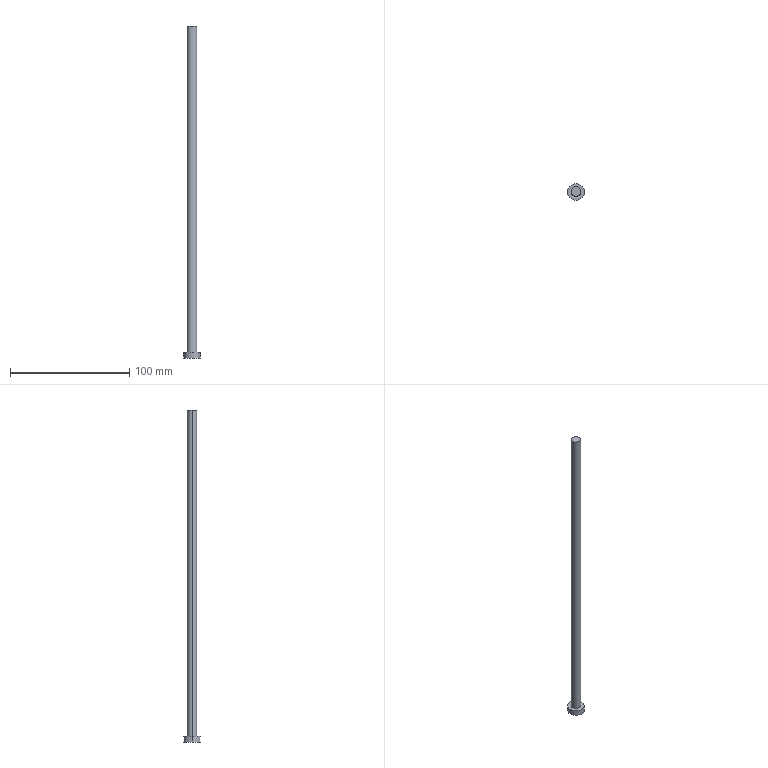Part | Creo | 1 solid | 7 faces | box 14 x 14 x 278.48 mm | volume 14516 mm3 | cylinder 4 | plane 3 | commonest cylinder face diameters 8 x2 14 x2
STEP:
#1=CARTESIAN_POINT('',(-176.,39.,42.98));
#2=VERTEX_POINT('',#1);
#3=CARTESIAN_POINT('',(-184.,39.,42.98));
#4=VERTEX_POINT('',#3);
#5=CARTESIAN_POINT('',(-180.,39.,42.98));
#6=DIRECTION('',(0.,0.,1.));
#7=DIRECTION('',(1.,0.,0.));
#8=AXIS2_PLACEMENT_3D('',#5,#6,#7);
#9=CIRCLE('',#8,4.);
#10=EDGE_CURVE('',#2,#4,#9,.T.);
#11=ORIENTED_EDGE('',*,*,#10,.T.);
#12=CARTESIAN_POINT('',(-184.,39.,-230.5));
#13=VERTEX_POINT('',#12);
#14=CARTESIAN_POINT('',(-184.,39.,42.98));
#15=DIRECTION('',(0.,0.,-1.));
#16=VECTOR('',#15,273.48);
#17=LINE('',#14,#16);
#18=EDGE_CURVE('',#4,#13,#17,.T.);
#19=ORIENTED_EDGE('',*,*,#18,.T.);
#20=CARTESIAN_POINT('',(-176.,39.,-230.5));
#21=VERTEX_POINT('',#20);
#22=CARTESIAN_POINT('',(-180.,39.,-230.5));
#23=DIRECTION('',(0.,0.,-1.));
#24=DIRECTION('',(-1.,0.,0.));
#25=AXIS2_PLACEMENT_3D('',#22,#23,#24);
#26=CIRCLE('',#25,4.);
#27=EDGE_CURVE('',#13,#21,#26,.T.);
#28=ORIENTED_EDGE('',*,*,#27,.T.);
#29=CARTESIAN_POINT('',(-176.,39.,42.98));
#30=DIRECTION('',(0.,0.,-1.));
#31=VECTOR('',#30,273.48);
#32=LINE('',#29,#31);
#33=EDGE_CURVE('',#2,#21,#32,.T.);
#34=ORIENTED_EDGE('',*,*,#33,.F.);
#35=EDGE_LOOP('',(#11,#19,#28,#34));
#36=FACE_OUTER_BOUND('',#35,.F.);
#37=CARTESIAN_POINT('',(-180.,39.,49.5));
#38=DIRECTION('',(0.,0.,-1.));
#39=DIRECTION('',(-1.,0.,0.));
#40=AXIS2_PLACEMENT_3D('',#37,#38,#39);
#41=CYLINDRICAL_SURFACE('',#40,4.);
#42=ADVANCED_FACE('',(#36),#41,.T.);
#43=CARTESIAN_POINT('',(-180.,39.,42.98));
#44=DIRECTION('',(0.,0.,1.));
#45=DIRECTION('',(-1.,0.,0.));
#46=AXIS2_PLACEMENT_3D('',#43,#44,#45);
#47=CIRCLE('',#46,4.);
#48=EDGE_CURVE('',#4,#2,#47,.T.);
#49=ORIENTED_EDGE('',*,*,#48,.F.);
#50=ORIENTED_EDGE('',*,*,#10,.F.);
#51=EDGE_LOOP('',(#49,#50));
#52=FACE_OUTER_BOUND('',#51,.F.);
#53=CARTESIAN_POINT('',(-179.214,-235.438,42.98));
#54=DIRECTION('',(0.,0.,-1.));
#55=DIRECTION('',(0.,1.,0.));
#56=AXIS2_PLACEMENT_3D('',#53,#54,#55);
#57=PLANE('',#56);
#58=ADVANCED_FACE('',(#52),#57,.F.);
#59=ORIENTED_EDGE('',*,*,#48,.T.);
#60=ORIENTED_EDGE('',*,*,#33,.T.);
#61=CARTESIAN_POINT('',(-180.,39.,-230.5));
#62=DIRECTION('',(0.,0.,-1.));
#63=DIRECTION('',(1.,0.,0.));
#64=AXIS2_PLACEMENT_3D('',#61,#62,#63);
#65=CIRCLE('',#64,4.);
#66=EDGE_CURVE('',#21,#13,#65,.T.);
#67=ORIENTED_EDGE('',*,*,#66,.T.);
#68=ORIENTED_EDGE('',*,*,#18,.F.);
#69=EDGE_LOOP('',(#59,#60,#67,#68));
#70=FACE_OUTER_BOUND('',#69,.F.);
#71=CARTESIAN_POINT('',(-180.,39.,49.5));
#72=DIRECTION('',(0.,0.,-1.));
#73=DIRECTION('',(-1.,0.,0.));
#74=AXIS2_PLACEMENT_3D('',#71,#72,#73);
#75=CYLINDRICAL_SURFACE('',#74,4.);
#76=ADVANCED_FACE('',(#70),#75,.T.);
#77=CARTESIAN_POINT('',(-187.,39.,-230.5));
#78=VERTEX_POINT('',#77);
#79=CARTESIAN_POINT('',(-173.,39.,-230.5));
#80=VERTEX_POINT('',#79);
#81=CARTESIAN_POINT('',(-180.,39.,-230.5));
#82=DIRECTION('',(0.,0.,1.));
#83=DIRECTION('',(-1.,0.,0.));
#84=AXIS2_PLACEMENT_3D('',#81,#82,#83);
#85=CIRCLE('',#84,7.);
#86=EDGE_CURVE('',#78,#80,#85,.T.);
#87=ORIENTED_EDGE('',*,*,#86,.F.);
#88=CARTESIAN_POINT('',(-180.,39.,-230.5));
#89=DIRECTION('',(0.,0.,1.));
#90=DIRECTION('',(1.,0.,0.));
#91=AXIS2_PLACEMENT_3D('',#88,#89,#90);
#92=CIRCLE('',#91,7.);
#93=EDGE_CURVE('',#80,#78,#92,.T.);
#94=ORIENTED_EDGE('',*,*,#93,.F.);
#95=EDGE_LOOP('',(#87,#94));
#96=FACE_OUTER_BOUND('',#95,.F.);
#97=ORIENTED_EDGE('',*,*,#27,.F.);
#98=ORIENTED_EDGE('',*,*,#66,.F.);
#99=EDGE_LOOP('',(#97,#98));
#100=FACE_BOUND('',#99,.F.);
#101=CARTESIAN_POINT('',(-180.,39.,-230.5));
#102=DIRECTION('',(0.,0.,-1.));
#103=DIRECTION('',(-1.,0.,0.));
#104=AXIS2_PLACEMENT_3D('',#101,#102,#103);
#105=PLANE('',#104);
#106=ADVANCED_FACE('',(#96,#100),#105,.F.);
#107=CARTESIAN_POINT('',(-173.,39.,-235.5));
#108=VERTEX_POINT('',#107);
#109=CARTESIAN_POINT('',(-187.,39.,-235.5));
#110=VERTEX_POINT('',#109);
#111=CARTESIAN_POINT('',(-180.,39.,-235.5));
#112=DIRECTION('',(0.,0.,-1.));
#113=DIRECTION('',(1.,0.,0.));
#114=AXIS2_PLACEMENT_3D('',#111,#112,#113);
#115=CIRCLE('',#114,7.);
#116=EDGE_CURVE('',#108,#110,#115,.T.);
#117=ORIENTED_EDGE('',*,*,#116,.T.);
#118=CARTESIAN_POINT('',(-187.,39.,-230.5));
#119=DIRECTION('',(0.,0.,-1.));
#120=VECTOR('',#119,5.);
#121=LINE('',#118,#120);
#122=EDGE_CURVE('',#78,#110,#121,.T.);
#123=ORIENTED_EDGE('',*,*,#122,.F.);
#124=ORIENTED_EDGE('',*,*,#86,.T.);
#125=CARTESIAN_POINT('',(-173.,39.,-230.5));
#126=DIRECTION('',(0.,0.,-1.));
#127=VECTOR('',#126,5.);
#128=LINE('',#125,#127);
#129=EDGE_CURVE('',#80,#108,#128,.T.);
#130=ORIENTED_EDGE('',*,*,#129,.T.);
#131=EDGE_LOOP('',(#117,#123,#124,#130));
#132=FACE_OUTER_BOUND('',#131,.F.);
#133=CARTESIAN_POINT('',(-180.,39.,-245.913));
#134=DIRECTION('',(0.,0.,-1.));
#135=DIRECTION('',(-1.,0.,0.));
#136=AXIS2_PLACEMENT_3D('',#133,#134,#135);
#137=CYLINDRICAL_SURFACE('',#136,7.);
#138=ADVANCED_FACE('',(#132),#137,.T.);
#139=CARTESIAN_POINT('',(-180.,39.,-235.5));
#140=DIRECTION('',(0.,0.,-1.));
#141=DIRECTION('',(-1.,0.,0.));
#142=AXIS2_PLACEMENT_3D('',#139,#140,#141);
#143=CIRCLE('',#142,7.);
#144=EDGE_CURVE('',#110,#108,#143,.T.);
#145=ORIENTED_EDGE('',*,*,#144,.F.);
#146=ORIENTED_EDGE('',*,*,#116,.F.);
#147=EDGE_LOOP('',(#145,#146));
#148=FACE_OUTER_BOUND('',#147,.F.);
#149=CARTESIAN_POINT('',(-176.,39.,-235.5));
#150=DIRECTION('',(0.,0.,1.));
#151=DIRECTION('',(1.,0.,0.));
#152=AXIS2_PLACEMENT_3D('',#149,#150,#151);
#153=PLANE('',#152);
#154=ADVANCED_FACE('',(#148),#153,.F.);
#155=ORIENTED_EDGE('',*,*,#144,.T.);
#156=ORIENTED_EDGE('',*,*,#129,.F.);
#157=ORIENTED_EDGE('',*,*,#93,.T.);
#158=ORIENTED_EDGE('',*,*,#122,.T.);
#159=EDGE_LOOP('',(#155,#156,#157,#158));
#160=FACE_OUTER_BOUND('',#159,.F.);
#161=CARTESIAN_POINT('',(-180.,39.,-245.913));
#162=DIRECTION('',(0.,0.,-1.));
#163=DIRECTION('',(-1.,0.,0.));
#164=AXIS2_PLACEMENT_3D('',#161,#162,#163);
#165=CYLINDRICAL_SURFACE('',#164,7.);
#166=ADVANCED_FACE('',(#160),#165,.T.);
#167=CLOSED_SHELL('',(#42,#58,#76,#106,#138,#154,#166));
#168=MANIFOLD_SOLID_BREP('',#167);
#169=(LENGTH_UNIT()NAMED_UNIT(*)SI_UNIT(.MILLI.,.METRE.));
#170=UNCERTAINTY_MEASURE_WITH_UNIT(LENGTH_MEASURE(0.02792),#169,'','');
#171=(NAMED_UNIT(*)PLANE_ANGLE_UNIT()SI_UNIT($,.RADIAN.));
#172=PLANE_ANGLE_MEASURE_WITH_UNIT(PLANE_ANGLE_MEASURE(0.01745),#171);
#173=(CONVERSION_BASED_UNIT('DEGREE',#172)NAMED_UNIT(*)PLANE_ANGLE_UNIT());
#174=(NAMED_UNIT(*)SI_UNIT($,.STERADIAN.)SOLID_ANGLE_UNIT());
#175=(GEOMETRIC_REPRESENTATION_CONTEXT(3)GLOBAL_UNCERTAINTY_ASSIGNED_CONTEXT((#170))GLOBAL_UNIT_ASSIGNED_CONTEXT((#169,#173,#174))REPRESENTATION_CONTEXT('',''));
#176=ADVANCED_BREP_SHAPE_REPRESENTATION('',(#168),#175);